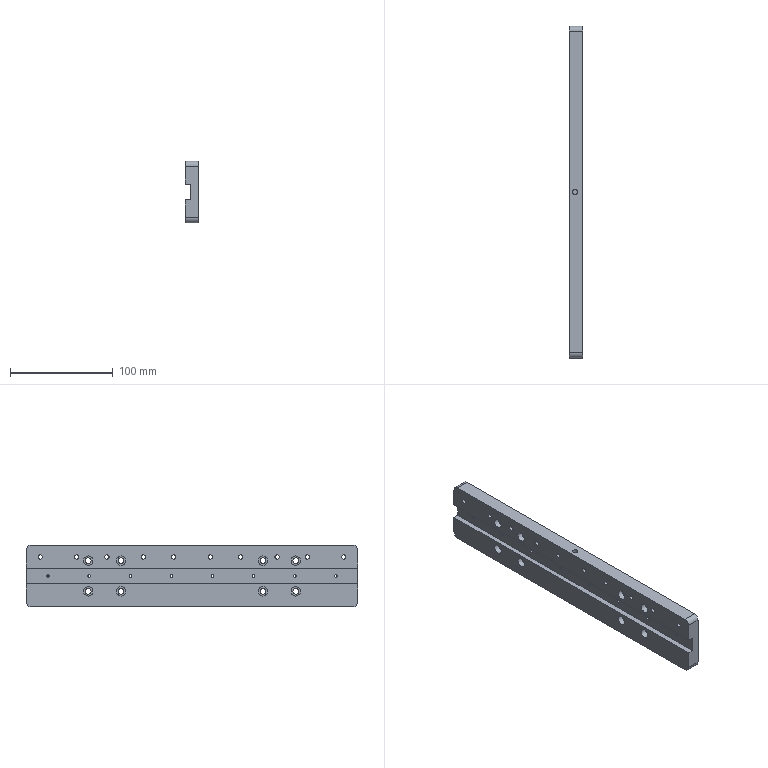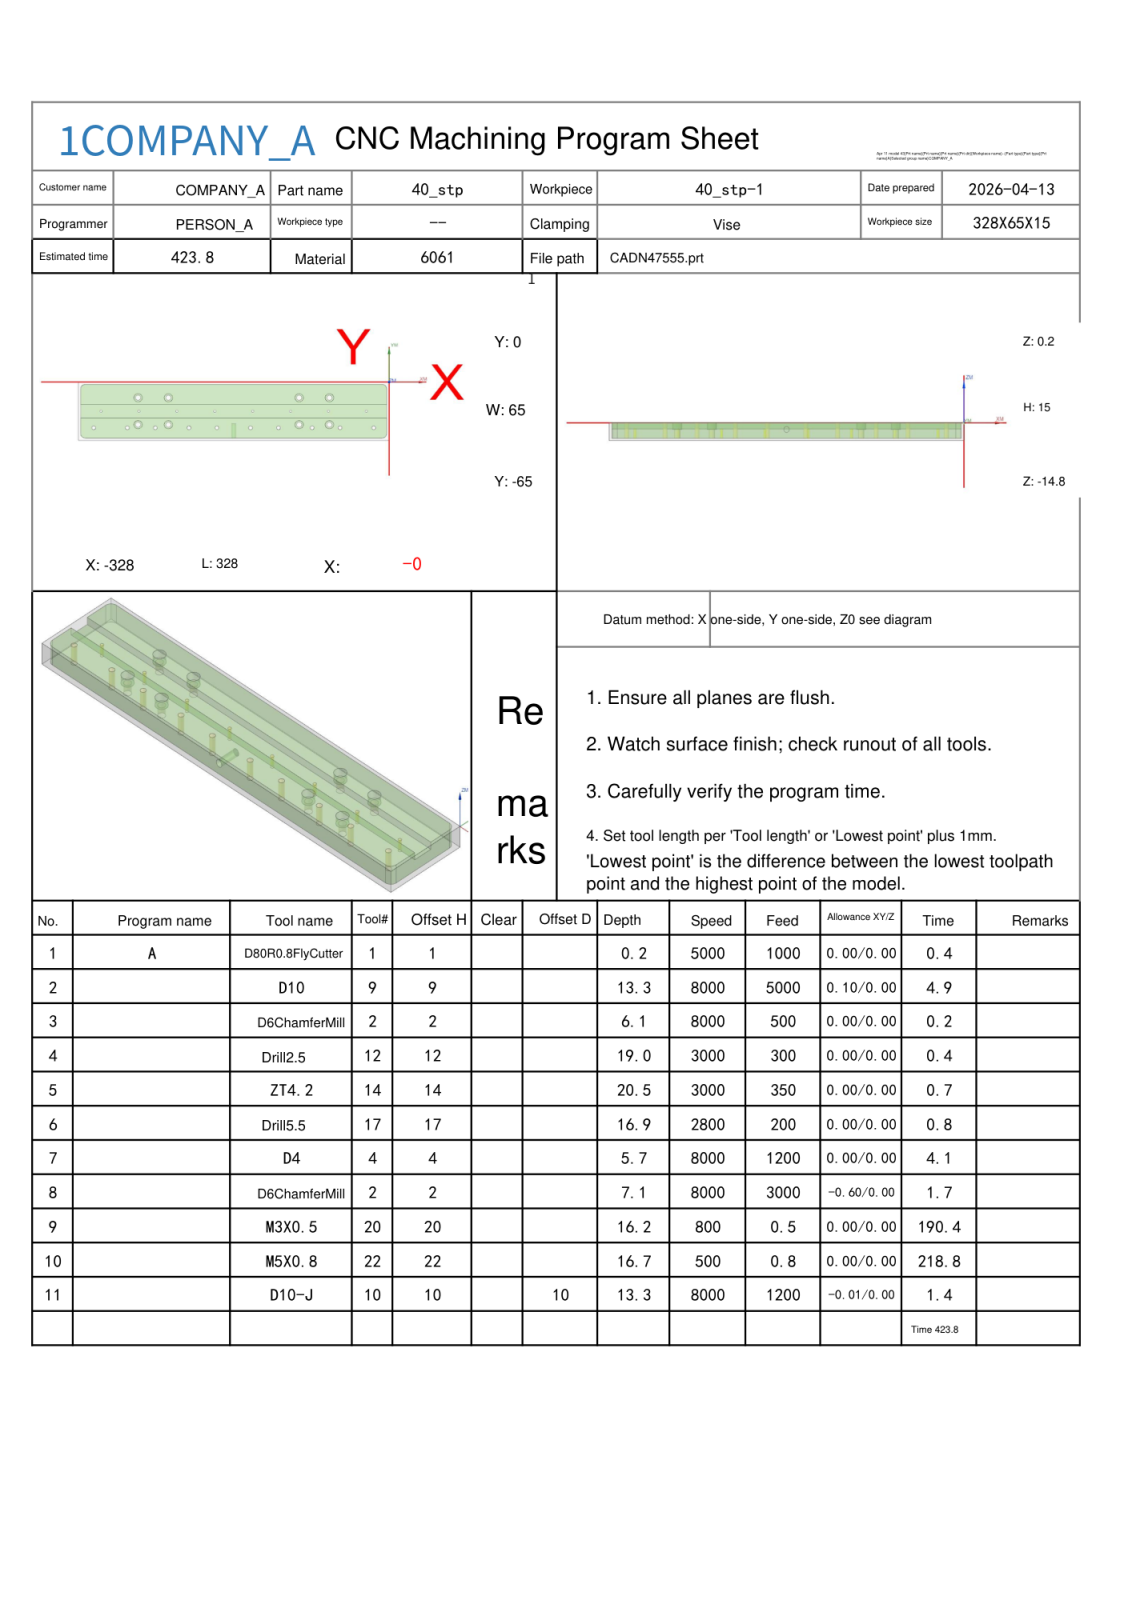NC program | NX | posted by the shop | part box 13 x 323 x 60 mm
Whole program, first 1421 of 1632 lines:
%
O0001
(Machine time: 806.56 MIN)
(===Total Tool:10===)
(T1=D80R0.8 FlyCutter D=80.  R=0.8  D-  H01 Z=-0.   )
(T9=D10     D=10.  R=0.   D-  H09 Z=-13.1 )
(T2=D6ChamferMill   D=6.   R=0.   D-  H02 Z=-6.85 )
(T12=Drill 2.5  D=2.5  DR_a=118 D-  H12 Z=-18.75)
(T14=ZT4.2  D=4.2  DR_a=118 D-  H14 Z=-20.26)
(T17=Drill 5.5  D=5.5  DR_a=118 D-  H17 Z=-16.65)
(T4=D4      D=4.   R=0.   D4  H04 Z=-5.5  )
(T20=M3X0.5 D=2.5  DR_a=180 D-  H20 Z=-16.  )
(T22=M5X0.8 D=4.2  DR_a=180 D-  H22 Z=-16.5 )
(T10=D10-J  D=10.  R=0.   D10 H10 Z=-13.1 )
G80 G90 G17 G49 G40
G91 G28 Z0
M01
N1 T01 M06
(D80R0.8 FlyCutter  D=80. R=0.8 H=01 ce=0.00 di=0.00)
G00 G90 G54 X-370.5 Y-32.5 M03 S5000
G43 H01 Z20.
M08
Z2.
G01 Z0.0 F1000.
X-365.5
X37.5
X42.5
Z2.
G00 Z20.
G91 G28 Z0.0
M05
M09
G91 G28 Z0.0
M01
N2 T09 M06
(D10  D=10. R=0. H=09 ce=0.10 di=0.00)
G00 G90 G54 X-164. Y2.6 M03 S8000
G43 H09 Z20.
M08
Z.5
G01 X-7.5 Z.35 F5000.
G02 X2.6 Y-7.5 Z.335 I0.0 J-10.1
G01 Y-57.5 Z.287
G02 X-7.5 Y-67.6 Z.272 I-10.1 J0.0
G01 X-320.5 Z-.028
G02 X-330.6 Y-57.5 Z-.043 I0.0 J10.1
G01 Y-7.5 Z-.091
G02 X-320.5 Y2.6 Z-.106 I10.1 J0.0
G01 X-7.5 Z-.405
G02 X2.6 Y-7.5 Z-.421 I0.0 J-10.1
G01 Y-57.5 Z-.468
G02 X-7.5 Y-67.6 Z-.484 I-10.1 J0.0
G01 X-320.5 Z-.783
G02 X-330.6 Y-57.5 Z-.798 I0.0 J10.1
G01 Y-7.5 Z-.846
G02 X-320.5 Y2.6 Z-.861 I10.1 J0.0
G01 X-7.5 Z-1.161
G02 X2.6 Y-7.5 Z-1.176 I0.0 J-10.1
G01 Y-57.5 Z-1.224
G02 X-7.5 Y-67.6 Z-1.239 I-10.1 J0.0
G01 X-320.5 Z-1.539
G02 X-330.6 Y-57.5 Z-1.554 I0.0 J10.1
G01 Y-7.5 Z-1.602
G02 X-320.5 Y2.6 Z-1.617 I10.1 J0.0
G01 X-7.5 Z-1.916
G02 X2.6 Y-7.5 Z-1.932 I0.0 J-10.1
G01 Y-57.5 Z-1.979
G02 X-7.5 Y-67.6 Z-1.995 I-10.1 J0.0
G01 X-320.5 Z-2.294
G02 X-330.6 Y-57.5 Z-2.309 I0.0 J10.1
G01 Y-7.5 Z-2.357
G02 X-320.5 Y2.6 Z-2.372 I10.1 J0.0
G01 X-7.5 Z-2.672
G02 X2.6 Y-7.5 Z-2.687 I0.0 J-10.1
G01 Y-57.5 Z-2.735
G02 X-7.5 Y-67.6 Z-2.75 I-10.1 J0.0
G01 X-320.5 Z-3.05
G02 X-330.6 Y-57.5 Z-3.065 I0.0 J10.1
G01 Y-7.5 Z-3.113
G02 X-320.5 Y2.6 Z-3.128 I10.1 J0.0
G01 X-7.5 Z-3.428
G02 X2.6 Y-7.5 Z-3.443 I0.0 J-10.1
G01 Y-57.5 Z-3.491
G02 X-7.5 Y-67.6 Z-3.506 I-10.1 J0.0
G01 X-320.5 Z-3.805
G02 X-330.6 Y-57.5 Z-3.821 I0.0 J10.1
G01 Y-7.5 Z-3.868
G02 X-320.5 Y2.6 Z-3.884 I10.1 J0.0
G01 X-7.5 Z-4.183
G02 X2.6 Y-7.5 Z-4.198 I0.0 J-10.1
G01 Y-57.5 Z-4.246
G02 X-7.5 Y-67.6 Z-4.261 I-10.1 J0.0
G01 X-320.5 Z-4.561
G02 X-330.6 Y-57.5 Z-4.576 I0.0 J10.1
G01 Y-7.5 Z-4.624
G02 X-320.5 Y2.6 Z-4.639 I10.1 J0.0
G01 X-7.5 Z-4.939
G02 X2.6 Y-7.5 Z-4.954 I0.0 J-10.1
G01 Y-57.5 Z-5.002
G02 X-7.5 Y-67.6 Z-5.017 I-10.1 J0.0
G01 X-320.5 Z-5.316
G02 X-330.6 Y-57.5 Z-5.332 I0.0 J10.1
G01 Y-7.5 Z-5.379
G02 X-320.5 Y2.6 Z-5.395 I10.1 J0.0
G01 X-7.5 Z-5.694
G02 X2.6 Y-7.5 Z-5.709 I0.0 J-10.1
G01 Y-57.5 Z-5.757
G02 X-7.5 Y-67.6 Z-5.772 I-10.1 J0.0
G01 X-320.5 Z-6.072
G02 X-330.6 Y-57.5 Z-6.087 I0.0 J10.1
G01 Y-7.5 Z-6.135
G02 X-320.5 Y2.6 Z-6.15 I10.1 J0.0
G01 X-7.5 Z-6.45
G02 X2.6 Y-7.5 Z-6.465 I0.0 J-10.1
G01 Y-57.5 Z-6.513
G02 X-7.5 Y-67.6 Z-6.528 I-10.1 J0.0
G01 X-320.5 Z-6.828
G02 X-330.6 Y-57.5 Z-6.843 I0.0 J10.1
G01 Y-7.5 Z-6.891
G02 X-320.5 Y2.6 Z-6.906 I10.1 J0.0
G01 X-7.5 Z-7.205
G02 X2.6 Y-7.5 Z-7.221 I0.0 J-10.1
G01 Y-57.5 Z-7.268
G02 X-7.5 Y-67.6 Z-7.284 I-10.1 J0.0
G01 X-320.5 Z-7.583
G02 X-330.6 Y-57.5 Z-7.598 I0.0 J10.1
G01 Y-7.5 Z-7.646
G02 X-320.5 Y2.6 Z-7.661 I10.1 J0.0
G01 X-7.5 Z-7.961
G02 X2.6 Y-7.5 Z-7.976 I0.0 J-10.1
G01 Y-57.5 Z-8.024
G02 X-7.5 Y-67.6 Z-8.039 I-10.1 J0.0
G01 X-320.5 Z-8.339
G02 X-330.6 Y-57.5 Z-8.354 I0.0 J10.1
G01 Y-7.5 Z-8.402
G02 X-320.5 Y2.6 Z-8.417 I10.1 J0.0
G01 X-7.5 Z-8.716
G02 X2.6 Y-7.5 Z-8.732 I0.0 J-10.1
G01 Y-57.5 Z-8.779
G02 X-7.5 Y-67.6 Z-8.795 I-10.1 J0.0
G01 X-320.5 Z-9.094
G02 X-330.6 Y-57.5 Z-9.109 I0.0 J10.1
G01 Y-7.5 Z-9.157
G02 X-320.5 Y2.6 Z-9.172 I10.1 J0.0
G01 X-7.5 Z-9.472
G02 X2.6 Y-7.5 Z-9.487 I0.0 J-10.1
G01 Y-57.5 Z-9.535
G02 X-7.5 Y-67.6 Z-9.55 I-10.1 J0.0
G01 X-320.5 Z-9.85
G02 X-330.6 Y-57.5 Z-9.865 I0.0 J10.1
G01 Y-7.5 Z-9.913
G02 X-320.5 Y2.6 Z-9.928 I10.1 J0.0
G01 X-7.5 Z-10.228
G02 X2.6 Y-7.5 Z-10.243 I0.0 J-10.1
G01 Y-57.5 Z-10.291
G02 X-7.5 Y-67.6 Z-10.306 I-10.1 J0.0
G01 X-320.5 Z-10.605
G02 X-330.6 Y-57.5 Z-10.621 I0.0 J10.1
G01 Y-7.5 Z-10.668
G02 X-320.5 Y2.6 Z-10.684 I10.1 J0.0
G01 X-7.5 Z-10.983
G02 X2.6 Y-7.5 Z-10.998 I0.0 J-10.1
G01 Y-57.5 Z-11.046
G02 X-7.5 Y-67.6 Z-11.061 I-10.1 J0.0
G01 X-320.5 Z-11.361
G02 X-330.6 Y-57.5 Z-11.376 I0.0 J10.1
G01 Y-7.5 Z-11.424
G02 X-320.5 Y2.6 Z-11.439 I10.1 J0.0
G01 X-7.5 Z-11.739
G02 X2.6 Y-7.5 Z-11.754 I0.0 J-10.1
G01 Y-57.5 Z-11.802
G02 X-7.5 Y-67.6 Z-11.817 I-10.1 J0.0
G01 X-320.5 Z-12.116
G02 X-330.6 Y-57.5 Z-12.132 I0.0 J10.1
G01 Y-7.5 Z-12.179
G02 X-320.5 Y2.6 Z-12.195 I10.1 J0.0
G01 X-7.5 Z-12.494
G02 X2.6 Y-7.5 Z-12.509 I0.0 J-10.1
G01 Y-57.5 Z-12.557
G02 X-7.5 Y-67.6 Z-12.572 I-10.1 J0.0
G01 X-320.5 Z-12.872
G02 X-330.6 Y-57.5 Z-12.887 I0.0 J10.1
G01 Y-7.5 Z-12.935
G02 X-320.5 Y2.6 Z-12.95 I10.1 J0.0
G01 X-164. Z-13.1
X-7.5
G02 X2.6 Y-7.5 I0.0 J-10.1
G01 Y-57.5
G02 X-7.5 Y-67.6 I-10.1 J0.0
G01 X-320.5
G02 X-330.6 Y-57.5 I0.0 J10.1
G01 Y-7.5
G02 X-320.5 Y2.6 I10.1 J0.0
G01 X-164.
X-163.5
Z-12.1
G00 Z20.
G00 G90 X-333.6 Y-32.5 M03 S6000
Z20.
Z0.0
G01 Z-.5 F3500.
X-326.5
Y-34.95
X-1.5
Y-30.05
X-326.5
Y-32.5
Y-33.
Z0.0
G00 Z.5
X-333.6 Y-32.5
Z-.5
G01 Z-1.
X-326.5
Y-34.95
X-1.5
Y-30.05
X-326.5
Y-32.5
Y-33.
Z-.5
G00 Z0.0
X-333.6 Y-32.5
Z-1.
G01 Z-1.5
X-326.5
Y-34.95
X-1.5
Y-30.05
X-326.5
Y-32.5
Y-33.
Z-1.
G00 Z-.5
X-333.6 Y-32.5
Z-1.5
G01 Z-2.
X-326.5
Y-34.95
X-1.5
Y-30.05
X-326.5
Y-32.5
Y-33.
Z-1.5
G00 Z-1.
X-333.6 Y-32.5
Z-2.
G01 Z-2.5
X-326.5
Y-34.95
X-1.5
Y-30.05
X-326.5
Y-32.5
Y-33.
Z-2.
G00 Z-1.5
X-333.6 Y-32.5
Z-2.5
G01 Z-3.
X-326.5
Y-34.95
X-1.5
Y-30.05
X-326.5
Y-32.5
Y-33.
Z-2.5
G00 Z-2.
X-333.6 Y-32.5
Z-3.
G01 Z-3.5
X-326.5
Y-34.95
X-1.5
Y-30.05
X-326.5
Y-32.5
Y-33.
Z-3.
G00 Z-2.5
X-333.6 Y-32.5
Z-3.5
G01 Z-4.
X-326.5
Y-34.95
X-1.5
Y-30.05
X-326.5
Y-32.5
Y-33.
Z-3.5
G00 Z-3.
X-333.6 Y-32.5
Z-4.
G01 Z-4.5
X-326.5
Y-34.95
X-1.5
Y-30.05
X-326.5
Y-32.5
Y-33.
Z-4.
G00 Z-3.5
X-333.6 Y-32.5
Z-4.5
G01 Z-5.
X-326.5
Y-34.95
X-1.5
Y-30.05
X-326.5
Y-32.5
Y-33.
Z-4.5
G00 Z20.
G91 G28 Z0.0
M05
M09
G91 G28 Z0.0
M01
N3 T02 M06
(D6ChamferMill  D=6. R=0. H=02 ce=0.00 di=0.10)
G00 G90 G54 X-104. Y-32.5 M03 S8000
G43 H02 Z20.
M08
G98 G81 X-104. Y-32.5 Z-5.9 R-4.1 F500.
X-95. Y-17.5 Z-.8 R1.
X-63.
X-64. Y-32.5 Z-5.9 R-4.1
X-24.
X-16.25 Y-51. Z-.8 R1.
X-51.75
X-63. Y-47.5
X-81.25 Y-51.
X-95. Y-47.5
X-116.75 Y-51.
X-146.25
X-144. Y-32.5 Z-5.9 R-4.1
X-184.
X-181.75 Y-51. Z-.8 R1.
X-211.25
X-233. Y-47.5
X-246.75 Y-51.
X-224. Y-32.5 Z-5.9 R-4.1
X-233. Y-17.5 Z-.8 R1.
X-265.
X-264. Y-32.5 Z-5.9 R-4.1
X-265. Y-47.5 Z-.8 R1.
X-276.25 Y-51.
X-311.75
X-304. Y-32.5 Z-5.9 R-4.1
G80
G00 Z20.
G91 G28 Z0.0
M05
M09
G91 G28 Z0.0
M01
N4 T12 M06
(Drill 2.5 D=2.5 DR_a=118 H=12)
G00 G90 G54 X-24. Y-32.5 M03 S3000
G43 H12 Z20.
M08
G98 G83 X-24. Y-32.5 Z-18.751 R-4.1 F300. Q2.
X-64.
X-104.
X-144.
X-184.
X-224.
X-264.
X-304.
G80
G00 Z20.
G91 G28 Z0.0
M05
M09
G91 G28 Z0.0
M01
N5 T14 M06
(ZT4.2 D=4.2 DR_a=118 H=14)
G00 G90 G54 X-16.25 Y-51. M03 S3000
G43 H14 Z20.
M08
G98 G83 X-16.25 Y-51. Z-20.262 R1. F350. Q3.
X-51.75
X-81.25
X-116.75
X-146.25
X-181.75
X-211.25
X-246.75
X-276.25
X-311.75
G80
G00 Z20.
G91 G28 Z0.0
M05
M09
G91 G28 Z0.0
M01
N6 T17 M06
(Drill 5.5 D=5.5 DR_a=118 H=17)
G00 G90 G54 X-63. Y-17.5 M03 S2800
G43 H17 Z20.
M08
G98 G83 X-63. Y-17.5 Z-16.652 R1. F200. Q2.
Y-47.5
X-95.
Y-17.5
X-233.
Y-47.5
X-265.
Y-17.5
G80
G00 Z20.
G91 G28 Z0.0
M05
M09
G91 G28 Z0.0
M01
N7 T04 M06
(D4  D=4. R=0. H=04 ce=0.10 di=0.00)
G00 G90 G54 X-63. Y-17.5 M03 S8000
G43 H04 Z20.
M08
Z.5
G03 X-62.4 Y-18.1 I.6 J0.0 F1200.
X-61.8 Y-17.5 I0.0 J.6
X-61.8 Y-17.5 Z.2 I-1.2 J0.0
X-61.8 Y-17.5 Z-.1 I-1.2 J0.0
X-61.8 Y-17.5 Z-.4 I-1.2 J0.0
X-61.8 Y-17.5 Z-.7 I-1.2 J0.0
X-61.8 Y-17.5 Z-1. I-1.2 J0.0
X-61.8 Y-17.5 Z-1.3 I-1.2 J0.0
X-61.8 Y-17.5 Z-1.6 I-1.2 J0.0
X-61.8 Y-17.5 Z-1.9 I-1.2 J0.0
X-61.8 Y-17.5 Z-2.2 I-1.2 J0.0
X-61.8 Y-17.5 Z-2.5 I-1.2 J0.0
X-61.8 Y-17.5 Z-2.8 I-1.2 J0.0
X-61.8 Y-17.5 Z-3.1 I-1.2 J0.0
X-61.8 Y-17.5 Z-3.4 I-1.2 J0.0
X-61.8 Y-17.5 Z-3.7 I-1.2 J0.0
X-61.8 Y-17.5 Z-4. I-1.2 J0.0
X-61.8 Y-17.5 Z-4.3 I-1.2 J0.0
X-61.8 Y-17.5 Z-4.6 I-1.2 J0.0
X-61.8 Y-17.5 Z-4.9 I-1.2 J0.0
X-61.8 Y-17.5 Z-5.2 I-1.2 J0.0
X-61.8 Y-17.5 Z-5.5 I-1.2 J0.0
X-63. Y-16.3 I-1.2 J0.0
X-64.2 Y-17.5 I0.0 J-1.2
X-63. Y-18.7 I1.2 J0.0
X-61.8 Y-17.5 I0.0 J1.2
X-62.4 Y-16.9 I-.6 J0.0
X-63. Y-17.5 I0.0 J-.6
G00 Z.5
G03 X-61.8 Y-18.7 I1.2 J0.0
X-60.6 Y-17.5 I0.0 J1.2
X-60.6 Y-17.5 Z.2 I-2.4 J0.0
X-60.6 Y-17.5 Z-.1 I-2.4 J0.0
X-60.6 Y-17.5 Z-.4 I-2.4 J0.0
X-60.6 Y-17.5 Z-.7 I-2.4 J0.0
X-60.6 Y-17.5 Z-1. I-2.4 J0.0
X-60.6 Y-17.5 Z-1.3 I-2.4 J0.0
X-60.6 Y-17.5 Z-1.6 I-2.4 J0.0
X-60.6 Y-17.5 Z-1.9 I-2.4 J0.0
X-60.6 Y-17.5 Z-2.2 I-2.4 J0.0
X-60.6 Y-17.5 Z-2.5 I-2.4 J0.0
X-60.6 Y-17.5 Z-2.8 I-2.4 J0.0
X-60.6 Y-17.5 Z-3.1 I-2.4 J0.0
X-60.6 Y-17.5 Z-3.4 I-2.4 J0.0
X-60.6 Y-17.5 Z-3.7 I-2.4 J0.0
X-60.6 Y-17.5 Z-4. I-2.4 J0.0
X-60.6 Y-17.5 Z-4.3 I-2.4 J0.0
X-60.6 Y-17.5 Z-4.6 I-2.4 J0.0
X-60.6 Y-17.5 Z-4.9 I-2.4 J0.0
X-60.6 Y-17.5 Z-5.2 I-2.4 J0.0
X-60.6 Y-17.5 Z-5.5 I-2.4 J0.0
X-63. Y-15.1 I-2.4 J0.0
X-65.4 Y-17.5 I0.0 J-2.4
X-63. Y-19.9 I2.4 J0.0
X-60.6 Y-17.5 I0.0 J2.4
X-61.8 Y-16.3 I-1.2 J0.0
X-63. Y-17.5 I0.0 J-1.2
G00 Z20.
Y-47.5
Z.5
G03 X-62.4 Y-48.1 I.6 J0.0
X-61.8 Y-47.5 I0.0 J.6
X-61.8 Y-47.5 Z.2 I-1.2 J0.0
X-61.8 Y-47.5 Z-.1 I-1.2 J0.0
X-61.8 Y-47.5 Z-.4 I-1.2 J0.0
X-61.8 Y-47.5 Z-.7 I-1.2 J0.0
X-61.8 Y-47.5 Z-1. I-1.2 J0.0
X-61.8 Y-47.5 Z-1.3 I-1.2 J0.0
X-61.8 Y-47.5 Z-1.6 I-1.2 J0.0
X-61.8 Y-47.5 Z-1.9 I-1.2 J0.0
X-61.8 Y-47.5 Z-2.2 I-1.2 J0.0
X-61.8 Y-47.5 Z-2.5 I-1.2 J0.0
X-61.8 Y-47.5 Z-2.8 I-1.2 J0.0
X-61.8 Y-47.5 Z-3.1 I-1.2 J0.0
X-61.8 Y-47.5 Z-3.4 I-1.2 J0.0
X-61.8 Y-47.5 Z-3.7 I-1.2 J0.0
X-61.8 Y-47.5 Z-4. I-1.2 J0.0
X-61.8 Y-47.5 Z-4.3 I-1.2 J0.0
X-61.8 Y-47.5 Z-4.6 I-1.2 J0.0
X-61.8 Y-47.5 Z-4.9 I-1.2 J0.0
X-61.8 Y-47.5 Z-5.2 I-1.2 J0.0
X-61.8 Y-47.5 Z-5.5 I-1.2 J0.0
X-63. Y-46.3 I-1.2 J0.0
X-64.2 Y-47.5 I0.0 J-1.2
X-63. Y-48.7 I1.2 J0.0
X-61.8 Y-47.5 I0.0 J1.2
X-62.4 Y-46.9 I-.6 J0.0
X-63. Y-47.5 I0.0 J-.6
G00 Z.5
G03 X-61.8 Y-48.7 I1.2 J0.0
X-60.6 Y-47.5 I0.0 J1.2
X-60.6 Y-47.5 Z.2 I-2.4 J0.0
X-60.6 Y-47.5 Z-.1 I-2.4 J0.0
X-60.6 Y-47.5 Z-.4 I-2.4 J0.0
X-60.6 Y-47.5 Z-.7 I-2.4 J0.0
X-60.6 Y-47.5 Z-1. I-2.4 J0.0
X-60.6 Y-47.5 Z-1.3 I-2.4 J0.0
X-60.6 Y-47.5 Z-1.6 I-2.4 J0.0
X-60.6 Y-47.5 Z-1.9 I-2.4 J0.0
X-60.6 Y-47.5 Z-2.2 I-2.4 J0.0
X-60.6 Y-47.5 Z-2.5 I-2.4 J0.0
X-60.6 Y-47.5 Z-2.8 I-2.4 J0.0
X-60.6 Y-47.5 Z-3.1 I-2.4 J0.0
X-60.6 Y-47.5 Z-3.4 I-2.4 J0.0
X-60.6 Y-47.5 Z-3.7 I-2.4 J0.0
X-60.6 Y-47.5 Z-4. I-2.4 J0.0
X-60.6 Y-47.5 Z-4.3 I-2.4 J0.0
X-60.6 Y-47.5 Z-4.6 I-2.4 J0.0
X-60.6 Y-47.5 Z-4.9 I-2.4 J0.0
X-60.6 Y-47.5 Z-5.2 I-2.4 J0.0
X-60.6 Y-47.5 Z-5.5 I-2.4 J0.0
X-63. Y-45.1 I-2.4 J0.0
X-65.4 Y-47.5 I0.0 J-2.4
X-63. Y-49.9 I2.4 J0.0
X-60.6 Y-47.5 I0.0 J2.4
X-61.8 Y-46.3 I-1.2 J0.0
X-63. Y-47.5 I0.0 J-1.2
G00 Z20.
X-95.
Z.5
G03 X-94.4 Y-48.1 I.6 J0.0
X-93.8 Y-47.5 I0.0 J.6
X-93.8 Y-47.5 Z.2 I-1.2 J0.0
X-93.8 Y-47.5 Z-.1 I-1.2 J0.0
X-93.8 Y-47.5 Z-.4 I-1.2 J0.0
X-93.8 Y-47.5 Z-.7 I-1.2 J0.0
X-93.8 Y-47.5 Z-1. I-1.2 J0.0
X-93.8 Y-47.5 Z-1.3 I-1.2 J0.0
X-93.8 Y-47.5 Z-1.6 I-1.2 J0.0
X-93.8 Y-47.5 Z-1.9 I-1.2 J0.0
X-93.8 Y-47.5 Z-2.2 I-1.2 J0.0
X-93.8 Y-47.5 Z-2.5 I-1.2 J0.0
X-93.8 Y-47.5 Z-2.8 I-1.2 J0.0
X-93.8 Y-47.5 Z-3.1 I-1.2 J0.0
X-93.8 Y-47.5 Z-3.4 I-1.2 J0.0
X-93.8 Y-47.5 Z-3.7 I-1.2 J0.0
X-93.8 Y-47.5 Z-4. I-1.2 J0.0
X-93.8 Y-47.5 Z-4.3 I-1.2 J0.0
X-93.8 Y-47.5 Z-4.6 I-1.2 J0.0
X-93.8 Y-47.5 Z-4.9 I-1.2 J0.0
X-93.8 Y-47.5 Z-5.2 I-1.2 J0.0
X-93.8 Y-47.5 Z-5.5 I-1.2 J0.0
X-95. Y-46.3 I-1.2 J0.0
X-96.2 Y-47.5 I0.0 J-1.2
X-95. Y-48.7 I1.2 J0.0
X-93.8 Y-47.5 I0.0 J1.2
X-94.4 Y-46.9 I-.6 J0.0
X-95. Y-47.5 I0.0 J-.6
G00 Z.5
G03 X-93.8 Y-48.7 I1.2 J0.0
X-92.6 Y-47.5 I0.0 J1.2
X-92.6 Y-47.5 Z.2 I-2.4 J0.0
X-92.6 Y-47.5 Z-.1 I-2.4 J0.0
X-92.6 Y-47.5 Z-.4 I-2.4 J0.0
X-92.6 Y-47.5 Z-.7 I-2.4 J0.0
X-92.6 Y-47.5 Z-1. I-2.4 J0.0
X-92.6 Y-47.5 Z-1.3 I-2.4 J0.0
X-92.6 Y-47.5 Z-1.6 I-2.4 J0.0
X-92.6 Y-47.5 Z-1.9 I-2.4 J0.0
X-92.6 Y-47.5 Z-2.2 I-2.4 J0.0
X-92.6 Y-47.5 Z-2.5 I-2.4 J0.0
X-92.6 Y-47.5 Z-2.8 I-2.4 J0.0
X-92.6 Y-47.5 Z-3.1 I-2.4 J0.0
X-92.6 Y-47.5 Z-3.4 I-2.4 J0.0
X-92.6 Y-47.5 Z-3.7 I-2.4 J0.0
X-92.6 Y-47.5 Z-4. I-2.4 J0.0
X-92.6 Y-47.5 Z-4.3 I-2.4 J0.0
X-92.6 Y-47.5 Z-4.6 I-2.4 J0.0
X-92.6 Y-47.5 Z-4.9 I-2.4 J0.0
X-92.6 Y-47.5 Z-5.2 I-2.4 J0.0
X-92.6 Y-47.5 Z-5.5 I-2.4 J0.0
X-95. Y-45.1 I-2.4 J0.0
X-97.4 Y-47.5 I0.0 J-2.4
X-95. Y-49.9 I2.4 J0.0
X-92.6 Y-47.5 I0.0 J2.4
X-93.8 Y-46.3 I-1.2 J0.0
X-95. Y-47.5 I0.0 J-1.2
G00 Z20.
Y-17.5
Z.5
G03 X-94.4 Y-18.1 I.6 J0.0
X-93.8 Y-17.5 I0.0 J.6
X-93.8 Y-17.5 Z.2 I-1.2 J0.0
X-93.8 Y-17.5 Z-.1 I-1.2 J0.0
X-93.8 Y-17.5 Z-.4 I-1.2 J0.0
X-93.8 Y-17.5 Z-.7 I-1.2 J0.0
X-93.8 Y-17.5 Z-1. I-1.2 J0.0
X-93.8 Y-17.5 Z-1.3 I-1.2 J0.0
X-93.8 Y-17.5 Z-1.6 I-1.2 J0.0
X-93.8 Y-17.5 Z-1.9 I-1.2 J0.0
X-93.8 Y-17.5 Z-2.2 I-1.2 J0.0
X-93.8 Y-17.5 Z-2.5 I-1.2 J0.0
X-93.8 Y-17.5 Z-2.8 I-1.2 J0.0
X-93.8 Y-17.5 Z-3.1 I-1.2 J0.0
X-93.8 Y-17.5 Z-3.4 I-1.2 J0.0
X-93.8 Y-17.5 Z-3.7 I-1.2 J0.0
X-93.8 Y-17.5 Z-4. I-1.2 J0.0
X-93.8 Y-17.5 Z-4.3 I-1.2 J0.0
X-93.8 Y-17.5 Z-4.6 I-1.2 J0.0
X-93.8 Y-17.5 Z-4.9 I-1.2 J0.0
X-93.8 Y-17.5 Z-5.2 I-1.2 J0.0
X-93.8 Y-17.5 Z-5.5 I-1.2 J0.0
X-95. Y-16.3 I-1.2 J0.0
X-96.2 Y-17.5 I0.0 J-1.2
X-95. Y-18.7 I1.2 J0.0
X-93.8 Y-17.5 I0.0 J1.2
X-94.4 Y-16.9 I-.6 J0.0
X-95. Y-17.5 I0.0 J-.6
G00 Z.5
G03 X-93.8 Y-18.7 I1.2 J0.0
X-92.6 Y-17.5 I0.0 J1.2
X-92.6 Y-17.5 Z.2 I-2.4 J0.0
X-92.6 Y-17.5 Z-.1 I-2.4 J0.0
X-92.6 Y-17.5 Z-.4 I-2.4 J0.0
X-92.6 Y-17.5 Z-.7 I-2.4 J0.0
X-92.6 Y-17.5 Z-1. I-2.4 J0.0
X-92.6 Y-17.5 Z-1.3 I-2.4 J0.0
X-92.6 Y-17.5 Z-1.6 I-2.4 J0.0
X-92.6 Y-17.5 Z-1.9 I-2.4 J0.0
X-92.6 Y-17.5 Z-2.2 I-2.4 J0.0
X-92.6 Y-17.5 Z-2.5 I-2.4 J0.0
X-92.6 Y-17.5 Z-2.8 I-2.4 J0.0
X-92.6 Y-17.5 Z-3.1 I-2.4 J0.0
X-92.6 Y-17.5 Z-3.4 I-2.4 J0.0
X-92.6 Y-17.5 Z-3.7 I-2.4 J0.0
X-92.6 Y-17.5 Z-4. I-2.4 J0.0
X-92.6 Y-17.5 Z-4.3 I-2.4 J0.0
X-92.6 Y-17.5 Z-4.6 I-2.4 J0.0
X-92.6 Y-17.5 Z-4.9 I-2.4 J0.0
X-92.6 Y-17.5 Z-5.2 I-2.4 J0.0
X-92.6 Y-17.5 Z-5.5 I-2.4 J0.0
X-95. Y-15.1 I-2.4 J0.0
X-97.4 Y-17.5 I0.0 J-2.4
X-95. Y-19.9 I2.4 J0.0
X-92.6 Y-17.5 I0.0 J2.4
X-93.8 Y-16.3 I-1.2 J0.0
X-95. Y-17.5 I0.0 J-1.2
G00 Z20.
X-233.
Z.5
G03 X-232.4 Y-18.1 I.6 J0.0
X-231.8 Y-17.5 I0.0 J.6
X-231.8 Y-17.5 Z.2 I-1.2 J0.0
X-231.8 Y-17.5 Z-.1 I-1.2 J0.0
X-231.8 Y-17.5 Z-.4 I-1.2 J0.0
X-231.8 Y-17.5 Z-.7 I-1.2 J0.0
X-231.8 Y-17.5 Z-1. I-1.2 J0.0
X-231.8 Y-17.5 Z-1.3 I-1.2 J0.0
X-231.8 Y-17.5 Z-1.6 I-1.2 J0.0
X-231.8 Y-17.5 Z-1.9 I-1.2 J0.0
X-231.8 Y-17.5 Z-2.2 I-1.2 J0.0
X-231.8 Y-17.5 Z-2.5 I-1.2 J0.0
X-231.8 Y-17.5 Z-2.8 I-1.2 J0.0
X-231.8 Y-17.5 Z-3.1 I-1.2 J0.0
X-231.8 Y-17.5 Z-3.4 I-1.2 J0.0
X-231.8 Y-17.5 Z-3.7 I-1.2 J0.0
X-231.8 Y-17.5 Z-4. I-1.2 J0.0
X-231.8 Y-17.5 Z-4.3 I-1.2 J0.0
X-231.8 Y-17.5 Z-4.6 I-1.2 J0.0
X-231.8 Y-17.5 Z-4.9 I-1.2 J0.0
X-231.8 Y-17.5 Z-5.2 I-1.2 J0.0
X-231.8 Y-17.5 Z-5.5 I-1.2 J0.0
X-233. Y-16.3 I-1.2 J0.0
X-234.2 Y-17.5 I0.0 J-1.2
X-233. Y-18.7 I1.2 J0.0
X-231.8 Y-17.5 I0.0 J1.2
X-232.4 Y-16.9 I-.6 J0.0
X-233. Y-17.5 I0.0 J-.6
G00 Z.5
G03 X-231.8 Y-18.7 I1.2 J0.0
X-230.6 Y-17.5 I0.0 J1.2
X-230.6 Y-17.5 Z.2 I-2.4 J0.0
X-230.6 Y-17.5 Z-.1 I-2.4 J0.0
X-230.6 Y-17.5 Z-.4 I-2.4 J0.0
X-230.6 Y-17.5 Z-.7 I-2.4 J0.0
X-230.6 Y-17.5 Z-1. I-2.4 J0.0
X-230.6 Y-17.5 Z-1.3 I-2.4 J0.0
X-230.6 Y-17.5 Z-1.6 I-2.4 J0.0
X-230.6 Y-17.5 Z-1.9 I-2.4 J0.0
X-230.6 Y-17.5 Z-2.2 I-2.4 J0.0
X-230.6 Y-17.5 Z-2.5 I-2.4 J0.0
X-230.6 Y-17.5 Z-2.8 I-2.4 J0.0
X-230.6 Y-17.5 Z-3.1 I-2.4 J0.0
X-230.6 Y-17.5 Z-3.4 I-2.4 J0.0
X-230.6 Y-17.5 Z-3.7 I-2.4 J0.0
X-230.6 Y-17.5 Z-4. I-2.4 J0.0
X-230.6 Y-17.5 Z-4.3 I-2.4 J0.0
X-230.6 Y-17.5 Z-4.6 I-2.4 J0.0
X-230.6 Y-17.5 Z-4.9 I-2.4 J0.0
X-230.6 Y-17.5 Z-5.2 I-2.4 J0.0
X-230.6 Y-17.5 Z-5.5 I-2.4 J0.0
X-233. Y-15.1 I-2.4 J0.0
X-235.4 Y-17.5 I0.0 J-2.4
X-233. Y-19.9 I2.4 J0.0
X-230.6 Y-17.5 I0.0 J2.4
X-231.8 Y-16.3 I-1.2 J0.0
X-233. Y-17.5 I0.0 J-1.2
G00 Z20.
Y-47.5
Z.5
G03 X-232.4 Y-48.1 I.6 J0.0
X-231.8 Y-47.5 I0.0 J.6
X-231.8 Y-47.5 Z.2 I-1.2 J0.0
X-231.8 Y-47.5 Z-.1 I-1.2 J0.0
X-231.8 Y-47.5 Z-.4 I-1.2 J0.0
X-231.8 Y-47.5 Z-.7 I-1.2 J0.0
X-231.8 Y-47.5 Z-1. I-1.2 J0.0
X-231.8 Y-47.5 Z-1.3 I-1.2 J0.0
X-231.8 Y-47.5 Z-1.6 I-1.2 J0.0
X-231.8 Y-47.5 Z-1.9 I-1.2 J0.0
X-231.8 Y-47.5 Z-2.2 I-1.2 J0.0
X-231.8 Y-47.5 Z-2.5 I-1.2 J0.0
X-231.8 Y-47.5 Z-2.8 I-1.2 J0.0
X-231.8 Y-47.5 Z-3.1 I-1.2 J0.0
X-231.8 Y-47.5 Z-3.4 I-1.2 J0.0
X-231.8 Y-47.5 Z-3.7 I-1.2 J0.0
X-231.8 Y-47.5 Z-4. I-1.2 J0.0
X-231.8 Y-47.5 Z-4.3 I-1.2 J0.0
X-231.8 Y-47.5 Z-4.6 I-1.2 J0.0
X-231.8 Y-47.5 Z-4.9 I-1.2 J0.0
X-231.8 Y-47.5 Z-5.2 I-1.2 J0.0
X-231.8 Y-47.5 Z-5.5 I-1.2 J0.0
X-233. Y-46.3 I-1.2 J0.0
X-234.2 Y-47.5 I0.0 J-1.2
X-233. Y-48.7 I1.2 J0.0
X-231.8 Y-47.5 I0.0 J1.2
X-232.4 Y-46.9 I-.6 J0.0
X-233. Y-47.5 I0.0 J-.6
G00 Z.5
G03 X-231.8 Y-48.7 I1.2 J0.0
X-230.6 Y-47.5 I0.0 J1.2
X-230.6 Y-47.5 Z.2 I-2.4 J0.0
X-230.6 Y-47.5 Z-.1 I-2.4 J0.0
X-230.6 Y-47.5 Z-.4 I-2.4 J0.0
X-230.6 Y-47.5 Z-.7 I-2.4 J0.0
X-230.6 Y-47.5 Z-1. I-2.4 J0.0
X-230.6 Y-47.5 Z-1.3 I-2.4 J0.0
X-230.6 Y-47.5 Z-1.6 I-2.4 J0.0
X-230.6 Y-47.5 Z-1.9 I-2.4 J0.0
X-230.6 Y-47.5 Z-2.2 I-2.4 J0.0
X-230.6 Y-47.5 Z-2.5 I-2.4 J0.0
X-230.6 Y-47.5 Z-2.8 I-2.4 J0.0
X-230.6 Y-47.5 Z-3.1 I-2.4 J0.0
X-230.6 Y-47.5 Z-3.4 I-2.4 J0.0
X-230.6 Y-47.5 Z-3.7 I-2.4 J0.0
X-230.6 Y-47.5 Z-4. I-2.4 J0.0
X-230.6 Y-47.5 Z-4.3 I-2.4 J0.0
X-230.6 Y-47.5 Z-4.6 I-2.4 J0.0
X-230.6 Y-47.5 Z-4.9 I-2.4 J0.0
X-230.6 Y-47.5 Z-5.2 I-2.4 J0.0
X-230.6 Y-47.5 Z-5.5 I-2.4 J0.0
X-233. Y-45.1 I-2.4 J0.0
X-235.4 Y-47.5 I0.0 J-2.4
X-233. Y-49.9 I2.4 J0.0
X-230.6 Y-47.5 I0.0 J2.4
X-231.8 Y-46.3 I-1.2 J0.0
X-233. Y-47.5 I0.0 J-1.2
G00 Z20.
X-265.
Z.5
G03 X-264.4 Y-48.1 I.6 J0.0
X-263.8 Y-47.5 I0.0 J.6
X-263.8 Y-47.5 Z.2 I-1.2 J0.0
X-263.8 Y-47.5 Z-.1 I-1.2 J0.0
X-263.8 Y-47.5 Z-.4 I-1.2 J0.0
X-263.8 Y-47.5 Z-.7 I-1.2 J0.0
X-263.8 Y-47.5 Z-1. I-1.2 J0.0
X-263.8 Y-47.5 Z-1.3 I-1.2 J0.0
X-263.8 Y-47.5 Z-1.6 I-1.2 J0.0
X-263.8 Y-47.5 Z-1.9 I-1.2 J0.0
X-263.8 Y-47.5 Z-2.2 I-1.2 J0.0
X-263.8 Y-47.5 Z-2.5 I-1.2 J0.0
X-263.8 Y-47.5 Z-2.8 I-1.2 J0.0
X-263.8 Y-47.5 Z-3.1 I-1.2 J0.0
X-263.8 Y-47.5 Z-3.4 I-1.2 J0.0
X-263.8 Y-47.5 Z-3.7 I-1.2 J0.0
X-263.8 Y-47.5 Z-4. I-1.2 J0.0
X-263.8 Y-47.5 Z-4.3 I-1.2 J0.0
X-263.8 Y-47.5 Z-4.6 I-1.2 J0.0
X-263.8 Y-47.5 Z-4.9 I-1.2 J0.0
X-263.8 Y-47.5 Z-5.2 I-1.2 J0.0
X-263.8 Y-47.5 Z-5.5 I-1.2 J0.0
X-265. Y-46.3 I-1.2 J0.0
X-266.2 Y-47.5 I0.0 J-1.2
X-265. Y-48.7 I1.2 J0.0
X-263.8 Y-47.5 I0.0 J1.2
X-264.4 Y-46.9 I-.6 J0.0
X-265. Y-47.5 I0.0 J-.6
G00 Z.5
G03 X-263.8 Y-48.7 I1.2 J0.0
X-262.6 Y-47.5 I0.0 J1.2
X-262.6 Y-47.5 Z.2 I-2.4 J0.0
X-262.6 Y-47.5 Z-.1 I-2.4 J0.0
X-262.6 Y-47.5 Z-.4 I-2.4 J0.0
X-262.6 Y-47.5 Z-.7 I-2.4 J0.0
X-262.6 Y-47.5 Z-1. I-2.4 J0.0
X-262.6 Y-47.5 Z-1.3 I-2.4 J0.0
X-262.6 Y-47.5 Z-1.6 I-2.4 J0.0
X-262.6 Y-47.5 Z-1.9 I-2.4 J0.0
X-262.6 Y-47.5 Z-2.2 I-2.4 J0.0
X-262.6 Y-47.5 Z-2.5 I-2.4 J0.0
X-262.6 Y-47.5 Z-2.8 I-2.4 J0.0
X-262.6 Y-47.5 Z-3.1 I-2.4 J0.0
X-262.6 Y-47.5 Z-3.4 I-2.4 J0.0
X-262.6 Y-47.5 Z-3.7 I-2.4 J0.0
X-262.6 Y-47.5 Z-4. I-2.4 J0.0
X-262.6 Y-47.5 Z-4.3 I-2.4 J0.0
X-262.6 Y-47.5 Z-4.6 I-2.4 J0.0
X-262.6 Y-47.5 Z-4.9 I-2.4 J0.0
X-262.6 Y-47.5 Z-5.2 I-2.4 J0.0
X-262.6 Y-47.5 Z-5.5 I-2.4 J0.0
X-265. Y-45.1 I-2.4 J0.0
X-267.4 Y-47.5 I0.0 J-2.4
X-265. Y-49.9 I2.4 J0.0
X-262.6 Y-47.5 I0.0 J2.4
X-263.8 Y-46.3 I-1.2 J0.0
X-265. Y-47.5 I0.0 J-1.2
G00 Z20.
Y-17.5
Z.5
G03 X-264.4 Y-18.1 I.6 J0.0
X-263.8 Y-17.5 I0.0 J.6
X-263.8 Y-17.5 Z.2 I-1.2 J0.0
X-263.8 Y-17.5 Z-.1 I-1.2 J0.0
X-263.8 Y-17.5 Z-.4 I-1.2 J0.0
X-263.8 Y-17.5 Z-.7 I-1.2 J0.0
X-263.8 Y-17.5 Z-1. I-1.2 J0.0
X-263.8 Y-17.5 Z-1.3 I-1.2 J0.0
X-263.8 Y-17.5 Z-1.6 I-1.2 J0.0
X-263.8 Y-17.5 Z-1.9 I-1.2 J0.0
X-263.8 Y-17.5 Z-2.2 I-1.2 J0.0
X-263.8 Y-17.5 Z-2.5 I-1.2 J0.0
X-263.8 Y-17.5 Z-2.8 I-1.2 J0.0
X-263.8 Y-17.5 Z-3.1 I-1.2 J0.0
X-263.8 Y-17.5 Z-3.4 I-1.2 J0.0
X-263.8 Y-17.5 Z-3.7 I-1.2 J0.0
X-263.8 Y-17.5 Z-4. I-1.2 J0.0
X-263.8 Y-17.5 Z-4.3 I-1.2 J0.0
X-263.8 Y-17.5 Z-4.6 I-1.2 J0.0
X-263.8 Y-17.5 Z-4.9 I-1.2 J0.0
X-263.8 Y-17.5 Z-5.2 I-1.2 J0.0
X-263.8 Y-17.5 Z-5.5 I-1.2 J0.0
X-265. Y-16.3 I-1.2 J0.0
X-266.2 Y-17.5 I0.0 J-1.2
X-265. Y-18.7 I1.2 J0.0
X-263.8 Y-17.5 I0.0 J1.2
X-264.4 Y-16.9 I-.6 J0.0
X-265. Y-17.5 I0.0 J-.6
G00 Z.5
G03 X-263.8 Y-18.7 I1.2 J0.0
X-262.6 Y-17.5 I0.0 J1.2
X-262.6 Y-17.5 Z.2 I-2.4 J0.0
X-262.6 Y-17.5 Z-.1 I-2.4 J0.0
X-262.6 Y-17.5 Z-.4 I-2.4 J0.0
X-262.6 Y-17.5 Z-.7 I-2.4 J0.0
X-262.6 Y-17.5 Z-1. I-2.4 J0.0
X-262.6 Y-17.5 Z-1.3 I-2.4 J0.0
X-262.6 Y-17.5 Z-1.6 I-2.4 J0.0
X-262.6 Y-17.5 Z-1.9 I-2.4 J0.0
X-262.6 Y-17.5 Z-2.2 I-2.4 J0.0
X-262.6 Y-17.5 Z-2.5 I-2.4 J0.0
X-262.6 Y-17.5 Z-2.8 I-2.4 J0.0
X-262.6 Y-17.5 Z-3.1 I-2.4 J0.0
X-262.6 Y-17.5 Z-3.4 I-2.4 J0.0
X-262.6 Y-17.5 Z-3.7 I-2.4 J0.0
X-262.6 Y-17.5 Z-4. I-2.4 J0.0
X-262.6 Y-17.5 Z-4.3 I-2.4 J0.0
X-262.6 Y-17.5 Z-4.6 I-2.4 J0.0
X-262.6 Y-17.5 Z-4.9 I-2.4 J0.0
X-262.6 Y-17.5 Z-5.2 I-2.4 J0.0
X-262.6 Y-17.5 Z-5.5 I-2.4 J0.0
X-265. Y-15.1 I-2.4 J0.0
X-267.4 Y-17.5 I0.0 J-2.4
X-265. Y-19.9 I2.4 J0.0
X-262.6 Y-17.5 I0.0 J2.4
X-263.8 Y-16.3 I-1.2 J0.0
X-265. Y-17.5 I0.0 J-1.2
G00 Z20.
G00 G90 X-63. Y-17.5 M03 S8000
Z20.
Z.5
G41 D04
G01 X-62.968 Y-17.697 F500.
G03 X-61.742 Y-18.742 I1.226 J.197
X-60.5 Y-17.5 I0.0 J1.242
X-60.5 Y-17.5 Z-4.5 I-2.5 J0.0
X-62.227 Y-15.122 Z-5.5 I-2.5 J0.0
X-63. Y-15. I-.773 J-2.378
X-65.5 Y-17.5 I0.0 J-2.5
X-63. Y-20. I2.5 J0.0
X-60.5 Y-17.5 I0.0 J2.5
X-62.227 Y-15.122 I-2.5 J0.0
X-62.611 Y-15.062 I-.384 J-1.181
X-63.853 Y-16.304 I0.0 J-1.242
X-63.178 Y-17.409 I1.242 J0.0
G01 G40 X-63. Y-17.5
G00 Z20.
Y-47.5
Z.5
G41 D04
G01 X-62.968 Y-47.697
G03 X-61.742 Y-48.742 I1.226 J.197
X-60.5 Y-47.5 I0.0 J1.242
X-60.5 Y-47.5 Z-4.5 I-2.5 J0.0
X-62.227 Y-45.122 Z-5.5 I-2.5 J0.0
X-63. Y-45. I-.773 J-2.378
X-65.5 Y-47.5 I0.0 J-2.5
X-63. Y-50. I2.5 J0.0
X-60.5 Y-47.5 I0.0 J2.5
X-62.227 Y-45.122 I-2.5 J0.0
X-62.611 Y-45.062 I-.384 J-1.181
X-63.853 Y-46.304 I0.0 J-1.242
X-63.178 Y-47.409 I1.242 J0.0
G01 G40 X-63. Y-47.5
G00 Z20.
X-95.
Z.5
G41 D04
G01 X-94.968 Y-47.697
G03 X-93.742 Y-48.742 I1.226 J.197
X-92.5 Y-47.5 I0.0 J1.242
X-92.5 Y-47.5 Z-4.5 I-2.5 J0.0
X-94.227 Y-45.122 Z-5.5 I-2.5 J0.0
X-95. Y-45. I-.773 J-2.378
X-97.5 Y-47.5 I0.0 J-2.5
X-95. Y-50. I2.5 J0.0
X-92.5 Y-47.5 I0.0 J2.5
X-94.227 Y-45.122 I-2.5 J0.0
X-94.611 Y-45.062 I-.384 J-1.181
X-95.853 Y-46.304 I0.0 J-1.242
X-95.178 Y-47.409 I1.242 J0.0
G01 G40 X-95. Y-47.5
G00 Z20.
Y-17.5
Z.5
G41 D04
G01 X-94.968 Y-17.697
G03 X-93.742 Y-18.742 I1.226 J.197
X-92.5 Y-17.5 I0.0 J1.242
X-92.5 Y-17.5 Z-4.5 I-2.5 J0.0
X-94.227 Y-15.122 Z-5.5 I-2.5 J0.0
X-95. Y-15. I-.773 J-2.378
X-97.5 Y-17.5 I0.0 J-2.5
X-95. Y-20. I2.5 J0.0
X-92.5 Y-17.5 I0.0 J2.5
X-94.227 Y-15.122 I-2.5 J0.0
X-94.611 Y-15.062 I-.384 J-1.181
X-95.853 Y-16.304 I0.0 J-1.242
X-95.178 Y-17.409 I1.242 J0.0
G01 G40 X-95. Y-17.5
G00 Z20.
X-233.
Z.5
G41 D04
G01 X-232.968 Y-17.697
G03 X-231.742 Y-18.742 I1.226 J.197
X-230.5 Y-17.5 I0.0 J1.242
X-230.5 Y-17.5 Z-4.5 I-2.5 J0.0
X-232.227 Y-15.122 Z-5.5 I-2.5 J0.0
X-233. Y-15. I-.773 J-2.378
X-235.5 Y-17.5 I0.0 J-2.5
X-233. Y-20. I2.5 J0.0
X-230.5 Y-17.5 I0.0 J2.5
X-232.227 Y-15.122 I-2.5 J0.0
X-232.611 Y-15.062 I-.384 J-1.181
X-233.853 Y-16.304 I0.0 J-1.242
X-233.178 Y-17.409 I1.242 J0.0
G01 G40 X-233. Y-17.5
G00 Z20.
Y-47.5
Z.5
G41 D04
G01 X-232.968 Y-47.697
G03 X-231.742 Y-48.742 I1.226 J.197
X-230.5 Y-47.5 I0.0 J1.242
X-230.5 Y-47.5 Z-4.5 I-2.5 J0.0
X-232.227 Y-45.122 Z-5.5 I-2.5 J0.0
X-233. Y-45. I-.773 J-2.378
X-235.5 Y-47.5 I0.0 J-2.5
X-233. Y-50. I2.5 J0.0
X-230.5 Y-47.5 I0.0 J2.5
X-232.227 Y-45.122 I-2.5 J0.0
X-232.611 Y-45.062 I-.384 J-1.181
X-233.853 Y-46.304 I0.0 J-1.242
X-233.178 Y-47.409 I1.242 J0.0
G01 G40 X-233. Y-47.5
G00 Z20.
X-265.
Z.5
G41 D04
G01 X-264.968 Y-47.697
G03 X-263.742 Y-48.742 I1.226 J.197
X-262.5 Y-47.5 I0.0 J1.242
X-262.5 Y-47.5 Z-4.5 I-2.5 J0.0
X-264.227 Y-45.122 Z-5.5 I-2.5 J0.0
X-265. Y-45. I-.773 J-2.378
X-267.5 Y-47.5 I0.0 J-2.5
X-265. Y-50. I2.5 J0.0
X-262.5 Y-47.5 I0.0 J2.5
X-264.227 Y-45.122 I-2.5 J0.0
X-264.611 Y-45.062 I-.384 J-1.181
X-265.853 Y-46.304 I0.0 J-1.242
X-265.178 Y-47.409 I1.242 J0.0
G01 G40 X-265. Y-47.5
G00 Z20.
Y-17.5
Z.5
G41 D04
G01 X-264.968 Y-17.697
G03 X-263.742 Y-18.742 I1.226 J.197
X-262.5 Y-17.5 I0.0 J1.242
X-262.5 Y-17.5 Z-4.5 I-2.5 J0.0
X-264.227 Y-15.122 Z-5.5 I-2.5 J0.0
X-265. Y-15. I-.773 J-2.378
X-267.5 Y-17.5 I0.0 J-2.5
X-265. Y-20. I2.5 J0.0
X-262.5 Y-17.5 I0.0 J2.5
X-264.227 Y-15.122 I-2.5 J0.0
X-264.611 Y-15.062 I-.384 J-1.181
X-265.853 Y-16.304 I0.0 J-1.242
X-265.178 Y-17.409 I1.242 J0.0
G01 G40 X-265. Y-17.5
G00 Z20.
G91 G28 Z0.0
M05
M09
G91 G28 Z0.0
M01
N8 T02 M06
(D6ChamferMill  D=6. R=0. H=02 ce=0.00 di=0.00)
G00 G90 G54 X-163.75 Y-27.078 M03 S8000
G43 H02 Z20.
M08
Z2.099
G01 Z-1.499 F3000.
G03 X-163.67 Y-26.778 I-.52 J.3
X-163.97 Y-26.258 I-.6 J0.0
G01 X-164. Y-26.25
X-325.5
G02 X-326.8 Y-24.95 I0.0 J1.3
G01 Y-7.5
G02 X-320.5 Y-1.2 I6.3 J0.0
G01 X-7.5
G02 X-1.2 Y-7.5 I0.0 J-6.3
G01 Y-24.95
G02 X-2.5 Y-26.25 I-1.3 J0.0
G01 X-164.
X-164.03 Y-26.258
G03 X-164.33 Y-26.778 I.3 J-.52
X-164.25 Y-27.078 I.6 J0.0
G01 Z2.099
G00 Z2.251
Y-37.922
Z2.099
G01 Z-1.499
G03 X-164.33 Y-38.222 I.52 J-.3
X-164.03 Y-38.742 I.6 J0.0
G01 X-164. Y-38.75
X-2.5
G02 X-1.2 Y-40.05 I0.0 J-1.3
G01 Y-57.5
G02 X-7.5 Y-63.8 I-6.3 J0.0
G01 X-320.5
G02 X-326.8 Y-57.5 I0.0 J6.3
G01 Y-40.05
G02 X-325.5 Y-38.75 I1.3 J0.0
G01 X-164.
X-163.97 Y-38.742
G03 X-163.67 Y-38.222 I-.3 J.52
X-163.75 Y-37.922 I-.6 J0.0
G01 Z2.099
G00 Z20.
X-327.545 Y-37.001
Z1.755
G01 Z-6.599
G03 X-327.275 Y-37.073 I.27 J.468
X-326.807 Y-36.803 I0.0 J.54
G01 X-326.8 Y-36.776
Y-28.224
X-326.807 Y-28.197
G03 X-327.275 Y-27.927 I-.468 J-.27
X-327.545 Y-27.999 I0.0 J-.54
G01 Z1.755
G00 Z20.
X-.455
Z1.755
G01 Z-6.599
G03 X-.725 Y-27.927 I-.27 J-.468
X-1.193 Y-28.197 I0.0 J-.54
G01 X-1.2 Y-28.224
Y-36.776
X-1.193 Y-36.803
G03 X-.725 Y-37.073 I.468 J.27
X-.455 Y-37.001 I0.0 J.54
G01 Z1.755
G00 Z20.
G00 G90 X-24. Y-32.5 M03 S8000
Z20.
G98 G81 X-24. Y-32.5 Z-6.85 R-2.1 F500.
X-64.
X-104.
X-144.
X-184.
X-224.
X-264.
X-304.
G80
G00 Z20.
G00 G90 X-312.444 Y-51.093 M03 S8000
Z20.
Z-.5
G01 Z-1. F500.
X-313.25 Y-51.2
G03 X-311.75 Y-52.7 I1.5 J0.0
X-310.05 Y-51. I0.0 J1.7
X-311.75 Y-49.3 I-1.7 J0.0
X-313.45 Y-51. I0.0 J-1.7
X-311.75 Y-52.7 I1.7 J0.0
X-310.25 Y-51.2 I0.0 J1.5
G01 X-311.056 Y-51.093
Z-.5
G00 Z20.
X-276.944
Z-.5
G01 Z-1.
X-277.75 Y-51.2
G03 X-276.25 Y-52.7 I1.5 J0.0
X-274.55 Y-51. I0.0 J1.7
X-276.25 Y-49.3 I-1.7 J0.0
X-277.95 Y-51. I0.0 J-1.7
X-276.25 Y-52.7 I1.7 J0.0
X-274.75 Y-51.2 I0.0 J1.5
G01 X-275.556 Y-51.093
Z-.5
G00 Z20.
X-247.444
Z-.5
G01 Z-1.
X-248.25 Y-51.2
G03 X-246.75 Y-52.7 I1.5 J0.0
X-245.05 Y-51. I0.0 J1.7
X-246.75 Y-49.3 I-1.7 J0.0
X-248.45 Y-51. I0.0 J-1.7
X-246.75 Y-52.7 I1.7 J0.0
X-245.25 Y-51.2 I0.0 J1.5
G01 X-246.056 Y-51.093
Z-.5
G00 Z20.
X-211.944
Z-.5
G01 Z-1.
X-212.75 Y-51.2
G03 X-211.25 Y-52.7 I1.5 J0.0
X-209.55 Y-51. I0.0 J1.7
X-211.25 Y-49.3 I-1.7 J0.0
X-212.95 Y-51. I0.0 J-1.7
X-211.25 Y-52.7 I1.7 J0.0
X-209.75 Y-51.2 I0.0 J1.5
G01 X-210.556 Y-51.093
Z-.5
G00 Z20.
X-182.444
Z-.5
G01 Z-1.
X-183.25 Y-51.2
G03 X-181.75 Y-52.7 I1.5 J0.0
X-180.05 Y-51. I0.0 J1.7
X-181.75 Y-49.3 I-1.7 J0.0
X-183.45 Y-51. I0.0 J-1.7
X-181.75 Y-52.7 I1.7 J0.0
X-180.25 Y-51.2 I0.0 J1.5
G01 X-181.056 Y-51.093
Z-.5
G00 Z20.
X-146.944
Z-.5
G01 Z-1.
X-147.75 Y-51.2
G03 X-146.25 Y-52.7 I1.5 J0.0
X-144.55 Y-51. I0.0 J1.7
X-146.25 Y-49.3 I-1.7 J0.0
X-147.95 Y-51. I0.0 J-1.7
X-146.25 Y-52.7 I1.7 J0.0
X-144.75 Y-51.2 I0.0 J1.5
G01 X-145.556 Y-51.093
Z-.5
G00 Z20.
X-117.444
Z-.5
G01 Z-1.
X-118.25 Y-51.2
G03 X-116.75 Y-52.7 I1.5 J0.0
X-115.05 Y-51. I0.0 J1.7
X-116.75 Y-49.3 I-1.7 J0.0
X-118.45 Y-51. I0.0 J-1.7
X-116.75 Y-52.7 I1.7 J0.0
X-115.25 Y-51.2 I0.0 J1.5
G01 X-116.056 Y-51.093
Z-.5
G00 Z20.
X-81.944
Z-.5
G01 Z-1.
X-82.75 Y-51.2
G03 X-81.25 Y-52.7 I1.5 J0.0
X-79.55 Y-51. I0.0 J1.7
X-81.25 Y-49.3 I-1.7 J0.0
X-82.95 Y-51. I0.0 J-1.7
X-81.25 Y-52.7 I1.7 J0.0
X-79.75 Y-51.2 I0.0 J1.5
G01 X-80.556 Y-51.093
Z-.5
G00 Z20.
X-52.444
Z-.5
G01 Z-1.
X-53.25 Y-51.2
G03 X-51.75 Y-52.7 I1.5 J0.0
X-50.05 Y-51. I0.0 J1.7
X-51.75 Y-49.3 I-1.7 J0.0
X-53.45 Y-51. I0.0 J-1.7
X-51.75 Y-52.7 I1.7 J0.0
X-50.25 Y-51.2 I0.0 J1.5
G01 X-51.056 Y-51.093
Z-.5
G00 Z20.
X-16.944
Z-.5
G01 Z-1.
X-17.75 Y-51.2
G03 X-16.25 Y-52.7 I1.5 J0.0
X-14.55 Y-51. I0.0 J1.7
X-16.25 Y-49.3 I-1.7 J0.0
X-17.95 Y-51. I0.0 J-1.7
X-16.25 Y-52.7 I1.7 J0.0
X-14.75 Y-51.2 I0.0 J1.5
G01 X-15.556 Y-51.093
Z-.5
G00 Z20.
G00 G90 X-267.181 Y-44.391 M03 S8000
Z20.
Z2.5
G01 X-267.367 Y-44.523 Z2.417 F500.
X-267.684 Y-44.806 Z2.262
X-267.968 Y-45.123 Z2.107
X-268.215 Y-45.469 Z1.953
X-268.366 Y-45.731 Z1.843
X-268.543 Y-46.118 Z1.688
X-268.675 Y-46.522 Z1.533
X-268.761 Y-46.939 Z1.378
X-268.801 Y-47.363 Z1.223
X-268.792 Y-47.788 Z1.068
X-268.736 Y-48.21 Z.913
X-268.633 Y-48.623 Z.758
X-268.485 Y-49.022 Z.604
X-268.293 Y-49.402 Z.449
X-268.06 Y-49.758 Z.294
X-267.789 Y-50.085 Z.139
X-267.483 Y-50.381 Z-.016
X-267.146 Y-50.64 Z-.171
X-266.781 Y-50.86 Z-.326
X-266.395 Y-51.038 Z-.48
X-265.991 Y-51.172 Z-.635
X-265.575 Y-51.259 Z-.79
X-265.151 Y-51.3 Z-.945
X-265. Z-1.
G03 X-261.2 Y-47.5 I0.0 J3.8
X-265. Y-43.7 I-3.8 J0.0
X-268.8 Y-47.5 I0.0 J-3.8
X-265. Y-51.3 I3.8 J0.0
X-264.501 Y-51.267 I0.0 J3.8
G01 Z1.5
G00 Z20.
X-267.181 Y-14.391
Z2.5
G01 X-267.367 Y-14.523 Z2.417
X-267.684 Y-14.806 Z2.262
X-267.968 Y-15.123 Z2.107
X-268.215 Y-15.469 Z1.953
X-268.366 Y-15.731 Z1.843
X-268.543 Y-16.118 Z1.688
X-268.675 Y-16.522 Z1.533
X-268.761 Y-16.939 Z1.378
X-268.801 Y-17.363 Z1.223
X-268.792 Y-17.788 Z1.068
X-268.736 Y-18.21 Z.913
X-268.633 Y-18.623 Z.758
X-268.485 Y-19.022 Z.604
X-268.293 Y-19.402 Z.449
X-268.06 Y-19.758 Z.294
X-267.789 Y-20.085 Z.139
X-267.483 Y-20.381 Z-.016
X-267.146 Y-20.64 Z-.171
X-266.781 Y-20.86 Z-.326
X-266.395 Y-21.038 Z-.48
X-265.991 Y-21.172 Z-.635
X-265.575 Y-21.259 Z-.79
X-265.151 Y-21.3 Z-.945
X-265. Z-1.
G03 X-261.2 Y-17.5 I0.0 J3.8
X-265. Y-13.7 I-3.8 J0.0
X-268.8 Y-17.5 I0.0 J-3.8
X-265. Y-21.3 I3.8 J0.0
X-264.501 Y-21.267 I0.0 J3.8
G01 Z1.5
G00 Z20.
X-235.181 Y-14.391
Z2.5
G01 X-235.367 Y-14.523 Z2.417
X-235.684 Y-14.806 Z2.262
X-235.968 Y-15.123 Z2.107
X-236.215 Y-15.469 Z1.953
X-236.366 Y-15.731 Z1.843
X-236.543 Y-16.118 Z1.688
X-236.675 Y-16.522 Z1.533
X-236.761 Y-16.939 Z1.378
X-236.801 Y-17.363 Z1.223
X-236.792 Y-17.788 Z1.068
X-236.736 Y-18.21 Z.913
X-236.633 Y-18.623 Z.758
X-236.485 Y-19.022 Z.604
X-236.293 Y-19.402 Z.449
X-236.06 Y-19.758 Z.294
X-235.789 Y-20.085 Z.139
X-235.483 Y-20.381 Z-.016
X-235.146 Y-20.64 Z-.171
X-234.781 Y-20.86 Z-.326
X-234.395 Y-21.038 Z-.48
X-233.991 Y-21.172 Z-.635
X-233.575 Y-21.259 Z-.79
X-233.151 Y-21.3 Z-.945
X-233. Z-1.
G03 X-229.2 Y-17.5 I0.0 J3.8
X-233. Y-13.7 I-3.8 J0.0
X-236.8 Y-17.5 I0.0 J-3.8
X-233. Y-21.3 I3.8 J0.0
X-232.501 Y-21.267 I0.0 J3.8
G01 Z1.5
G00 Z20.
X-235.181 Y-44.391
Z2.5
G01 X-235.367 Y-44.523 Z2.417
X-235.684 Y-44.806 Z2.262
X-235.968 Y-45.123 Z2.107
X-236.215 Y-45.469 Z1.953
X-236.366 Y-45.731 Z1.843
X-236.543 Y-46.118 Z1.688
X-236.675 Y-46.522 Z1.533
X-236.761 Y-46.939 Z1.378
X-236.801 Y-47.363 Z1.223
X-236.792 Y-47.788 Z1.068
X-236.736 Y-48.21 Z.913
X-236.633 Y-48.623 Z.758
X-236.485 Y-49.022 Z.604
X-236.293 Y-49.402 Z.449
X-236.06 Y-49.758 Z.294
X-235.789 Y-50.085 Z.139
X-235.483 Y-50.381 Z-.016
X-235.146 Y-50.64 Z-.171
X-234.781 Y-50.86 Z-.326
X-234.395 Y-51.038 Z-.48
X-233.991 Y-51.172 Z-.635
X-233.575 Y-51.259 Z-.79
X-233.151 Y-51.3 Z-.945
X-233. Z-1.
G03 X-229.2 Y-47.5 I0.0 J3.8
X-233. Y-43.7 I-3.8 J0.0
X-236.8 Y-47.5 I0.0 J-3.8
X-233. Y-51.3 I3.8 J0.0
X-232.501 Y-51.267 I0.0 J3.8
G01 Z1.5
G00 Z20.
X-97.181 Y-44.391
Z2.5
G01 X-97.367 Y-44.523 Z2.417
X-97.684 Y-44.806 Z2.262
X-97.968 Y-45.123 Z2.107
X-98.215 Y-45.469 Z1.953
X-98.366 Y-45.731 Z1.843
X-98.543 Y-46.118 Z1.688
X-98.675 Y-46.522 Z1.533
X-98.761 Y-46.939 Z1.378
X-98.801 Y-47.363 Z1.223
X-98.792 Y-47.788 Z1.068
X-98.736 Y-48.21 Z.913
X-98.633 Y-48.623 Z.758
X-98.485 Y-49.022 Z.604
X-98.293 Y-49.402 Z.449
X-98.06 Y-49.758 Z.294
X-97.789 Y-50.085 Z.139
X-97.483 Y-50.381 Z-.016
X-97.146 Y-50.64 Z-.171